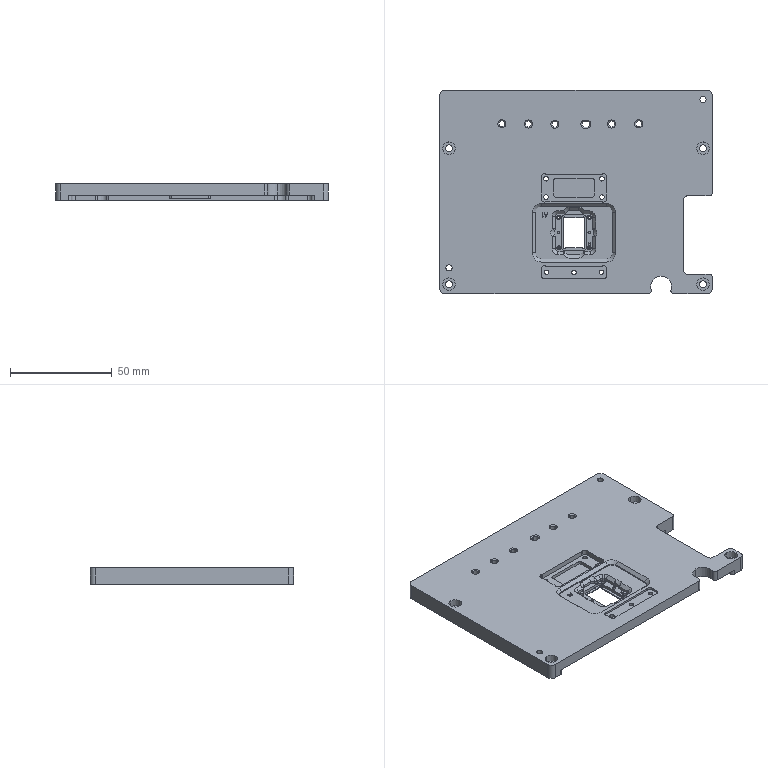Part | 1 solid | 570 faces | box 134 x 100 x 8 mm | volume 69429 mm3 | plane 222 | cylinder 210 | spline 99 | cone 39 | commonest cylinder face diameters 3 x32 3.5 x24 0.6 x15 2.2 x14 1 x12 3.4 x12